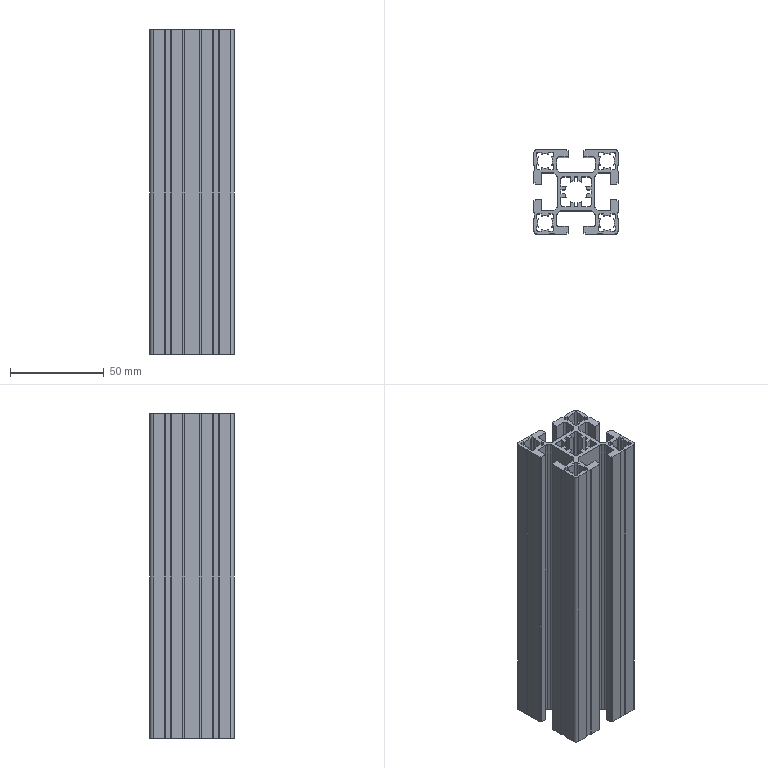Part | STEP file | 4545 aluminium computer rack upper cross | 1 solid | 262 faces | box 45 x 45 x 172.5 mm | volume 119689 mm3 | plane 186 | cylinder 76 | commonest cylinder face diameters 2 x44 8 x20 12 x8 4 x4